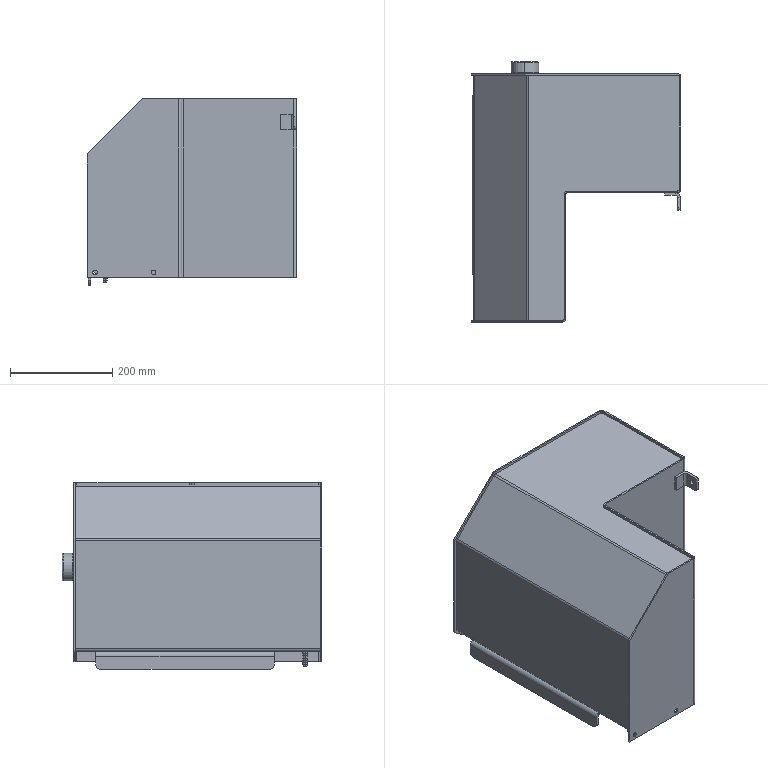Part | SolidWorks | features CompositeCurve 2 | 7 solids | 271 faces | box 410 x 509 x 365 mm | volume 2578736 mm3 | plane 122 | cylinder 108 | cone 19 | torus 16 | spline 6 | commonest cylinder face diameters 22 x14 6 x13 3.3 x12 12 x9 9 x8 10 x6